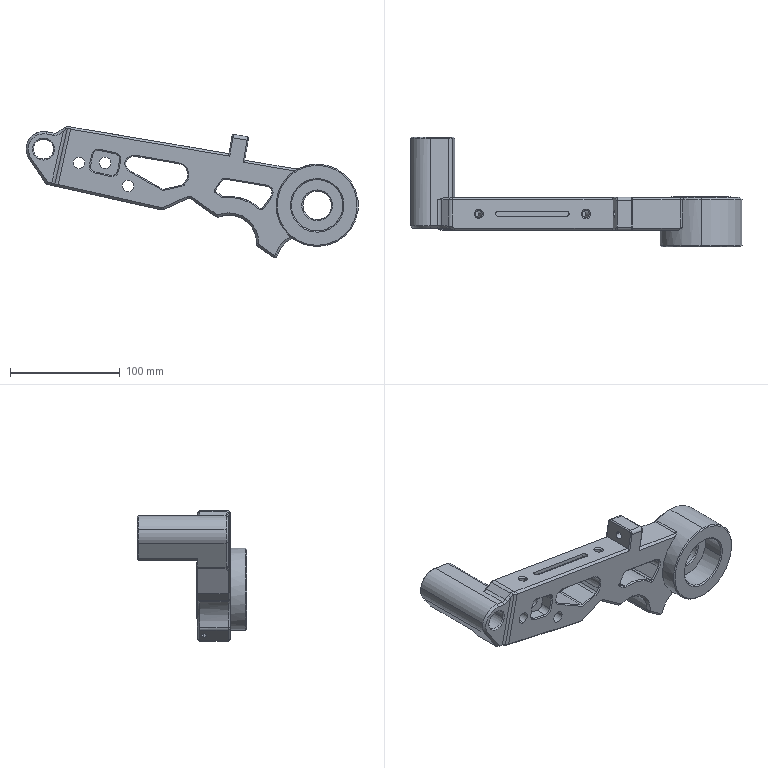Part | SolidWorks | features BaseBody 1 | 1 solid | 256 faces | box 302.851 x 100 x 119.199 mm | volume 509572 mm3 | cone 85 | plane 82 | cylinder 80 | spline 5 | torus 4 | commonest cylinder face diameters 10 x12 6 x10 2 x7 6.5 x6 10.5 x6 18 x6